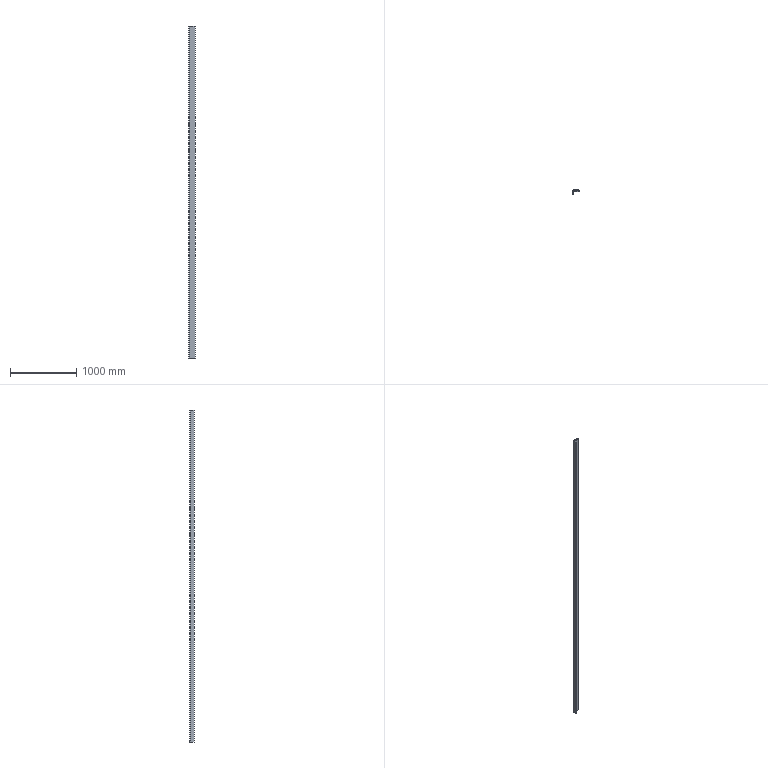Part | SolidWorks | features ICE 3, Extrusion 1, LPattern 1, MirrorPattern 1 | 1 solid | 116 faces | box 100 x 62 x 5000 mm | volume 12959941 mm3 | plane 116